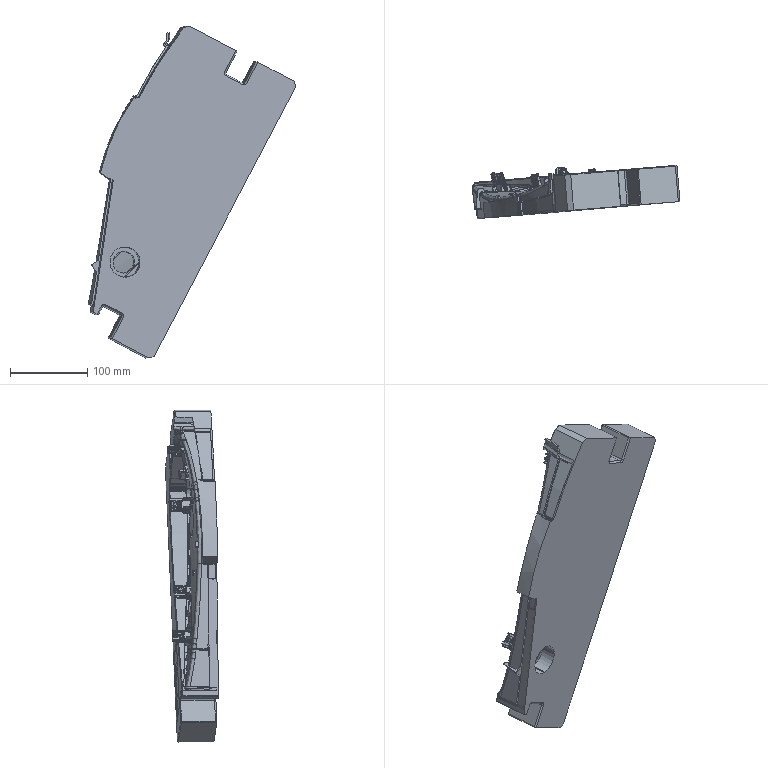Part | SolidWorks | features AEMSimFeature 1 | 5 solids | 3695 faces | volume 2042090 mm3 | spline 1955 | plane 985 | cylinder 745 | cone 10 | commonest cylinder face diameters 1 x303 0.6 x100 2 x77 1.8 x72 0.5 x44 0.4 x33